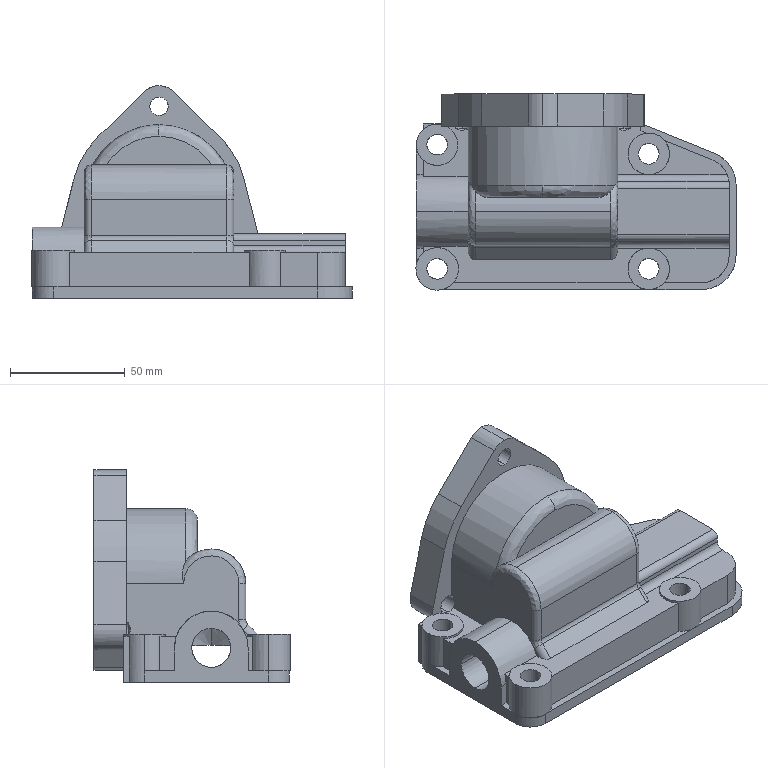Part | SolidWorks | features BaseBody 1 | 1 solid | 255 faces | box 139.25 x 85.25 x 92.5 mm | volume 171362 mm3 | cylinder 158 | plane 80 | spline 12 | cone 5 | commonest cylinder face diameters 9 x24 18 x21 8 x18 6 x16 17 x9 32 x9